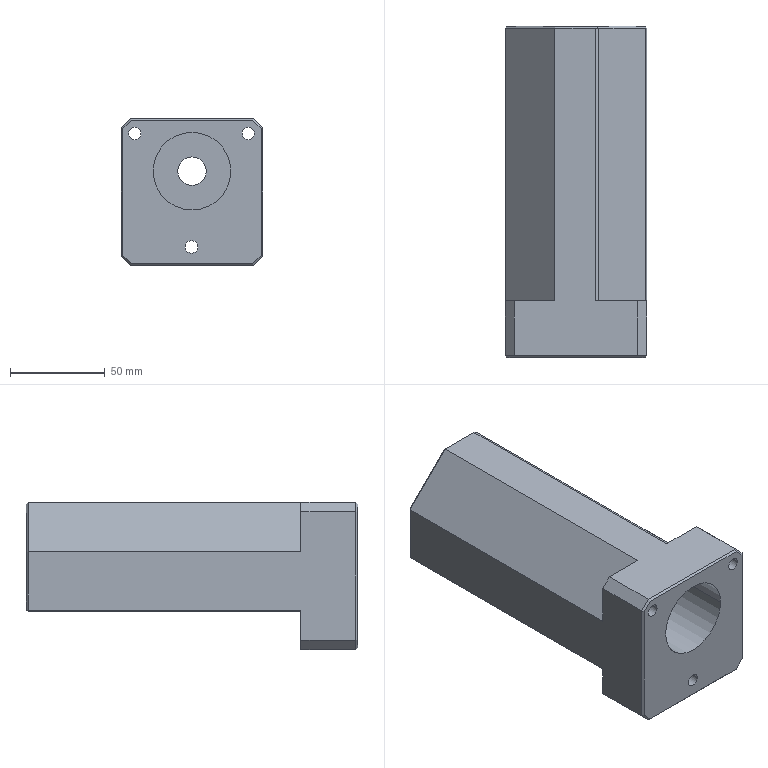Part | Creo | 1 solid | 58 faces | box 75 x 175 x 78 mm | volume 480642 mm3 | plane 42 | cylinder 16 | commonest cylinder face diameters 6.6 x6 11 x6 15 x2 41 x2